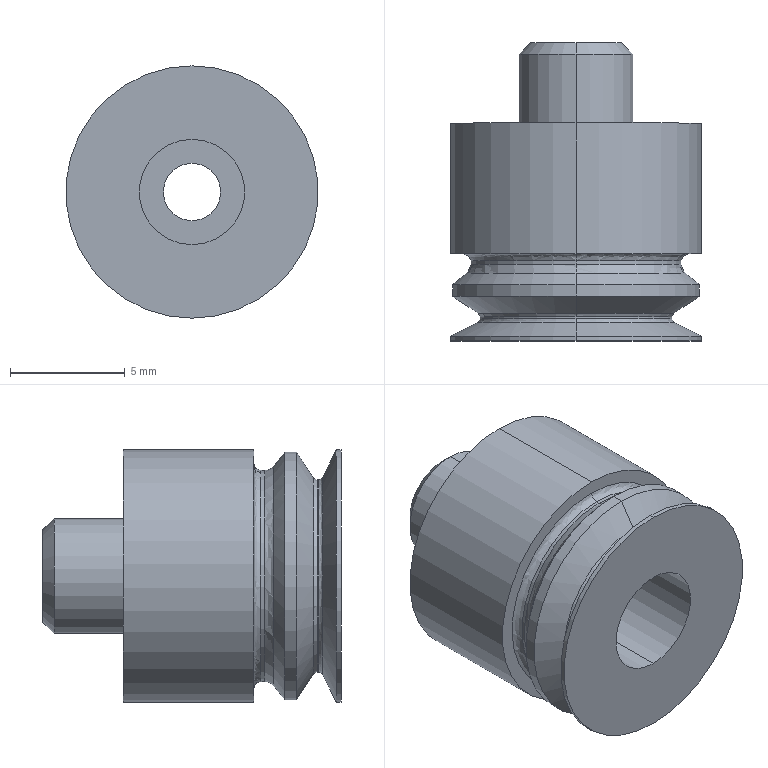Part | SolidWorks | features BaseBody 1 | 1 solid | 37 faces | box 11 x 13 x 11 mm | volume 720.123 mm3 | cylinder 16 | spline 8 | cone 8 | plane 5 | commonest cylinder face diameters 11 x4 2.5 x2 4.6 x2 5 x2 8.4 x2 9.2 x2
STEP:
#1=CARTESIAN_POINT('',(0.,-9.2,4.9));
#2=VERTEX_POINT('',#1);
#3=CARTESIAN_POINT('',(0.,-9.2,-4.9));
#4=VERTEX_POINT('',#3);
#5=CARTESIAN_POINT('',(0.,-9.2,4.9));
#6=CARTESIAN_POINT('',(0.3114,-9.2,4.9));
#7=CARTESIAN_POINT('',(0.7704,-9.2,4.857));
#8=CARTESIAN_POINT('',(1.292,-9.2,4.732));
#9=CARTESIAN_POINT('',(1.549,-9.2,4.65));
#10=CARTESIAN_POINT('',(1.677,-9.2,4.605));
#11=CARTESIAN_POINT('',(1.731,-9.2,4.584));
#12=CARTESIAN_POINT('',(1.767,-9.2,4.57));
#13=CARTESIAN_POINT('',(1.784,-9.2,4.564));
#14=CARTESIAN_POINT('',(1.957,-9.2,4.495));
#15=CARTESIAN_POINT('',(2.183,-9.2,4.393));
#16=CARTESIAN_POINT('',(2.399,-9.2,4.273));
#17=CARTESIAN_POINT('',(2.542,-9.2,4.19));
#18=CARTESIAN_POINT('',(2.611,-9.2,4.147));
#19=CARTESIAN_POINT('',(2.964,-9.2,3.916));
#20=CARTESIAN_POINT('',(3.226,-9.2,3.704));
#21=CARTESIAN_POINT('',(3.584,-9.2,3.345));
#22=CARTESIAN_POINT('',(3.753,-9.2,3.158));
#23=CARTESIAN_POINT('',(3.908,-9.2,2.958));
#24=CARTESIAN_POINT('',(4.007,-9.2,2.822));
#25=CARTESIAN_POINT('',(4.056,-9.2,2.751));
#26=CARTESIAN_POINT('',(4.192,-9.2,2.543));
#27=CARTESIAN_POINT('',(4.317,-9.2,2.329));
#28=CARTESIAN_POINT('',(4.443,-9.2,2.07));
#29=CARTESIAN_POINT('',(4.501,-9.2,1.938));
#30=CARTESIAN_POINT('',(4.525,-9.2,1.88));
#31=CARTESIAN_POINT('',(4.541,-9.2,1.842));
#32=CARTESIAN_POINT('',(4.549,-9.2,1.822));
#33=CARTESIAN_POINT('',(4.785,-9.2,1.225));
#34=CARTESIAN_POINT('',(4.9,-9.2,0.6227));
#35=CARTESIAN_POINT('',(4.9,-9.2,-0.3114));
#36=CARTESIAN_POINT('',(4.857,-9.2,-0.7704));
#37=CARTESIAN_POINT('',(4.732,-9.2,-1.292));
#38=CARTESIAN_POINT('',(4.65,-9.2,-1.549));
#39=CARTESIAN_POINT('',(4.605,-9.2,-1.677));
#40=CARTESIAN_POINT('',(4.584,-9.2,-1.731));
#41=CARTESIAN_POINT('',(4.57,-9.2,-1.767));
#42=CARTESIAN_POINT('',(4.564,-9.2,-1.784));
#43=CARTESIAN_POINT('',(4.495,-9.2,-1.957));
#44=CARTESIAN_POINT('',(4.393,-9.2,-2.183));
#45=CARTESIAN_POINT('',(4.273,-9.2,-2.399));
#46=CARTESIAN_POINT('',(4.19,-9.2,-2.542));
#47=CARTESIAN_POINT('',(4.147,-9.2,-2.611));
#48=CARTESIAN_POINT('',(3.916,-9.2,-2.964));
#49=CARTESIAN_POINT('',(3.704,-9.2,-3.226));
#50=CARTESIAN_POINT('',(3.345,-9.2,-3.584));
#51=CARTESIAN_POINT('',(3.158,-9.2,-3.753));
#52=CARTESIAN_POINT('',(2.958,-9.2,-3.908));
#53=CARTESIAN_POINT('',(2.822,-9.2,-4.007));
#54=CARTESIAN_POINT('',(2.751,-9.2,-4.056));
#55=CARTESIAN_POINT('',(2.543,-9.2,-4.192));
#56=CARTESIAN_POINT('',(2.329,-9.2,-4.317));
#57=CARTESIAN_POINT('',(2.07,-9.2,-4.443));
#58=CARTESIAN_POINT('',(1.957,-9.2,-4.493));
#59=CARTESIAN_POINT('',(1.88,-9.2,-4.525));
#60=CARTESIAN_POINT('',(1.841,-9.2,-4.541));
#61=CARTESIAN_POINT('',(1.656,-9.2,-4.614));
#62=CARTESIAN_POINT('',(1.431,-9.2,-4.691));
#63=CARTESIAN_POINT('',(1.163,-9.2,-4.761));
#64=CARTESIAN_POINT('',(1.028,-9.2,-4.791));
#65=CARTESIAN_POINT('',(0.9697,-9.2,-4.803));
#66=CARTESIAN_POINT('',(0.9307,-9.2,-4.811));
#67=CARTESIAN_POINT('',(0.91,-9.2,-4.815));
#68=CARTESIAN_POINT('',(0.5971,-9.2,-4.873));
#69=CARTESIAN_POINT('',(0.2999,-9.2,-4.9));
#70=CARTESIAN_POINT('',(0.,-9.2,-4.9));
#71=B_SPLINE_CURVE_WITH_KNOTS('',3,(#5,#6,#7,#8,#9,#10,#11,#12,#13,#14,#15,#16,#17,#18,#19,#20,#21,#22,#23,#24,#25,#26,#27,#28,#29,#30,#31,#32,#33,#34,#35,#36,#37,#38,#39,#40,#41,#42,#43,#44,#45,#46,#47,#48,#49,#50,#51,#52,#53,#54,#55,#56,#57,#58,#59,#60,#61,#62,#63,#64,#65,#66,#67,#68,#69,#70),.UNSPECIFIED.,.F.,.F.,(4,1,1,1,1,2,2,1,2,2,2,1,2,2,1,1,1,2,2,2,1,1,1,1,2,2,1,2,2,2,1,2,2,1,1,2,2,1,1,1,2,2,4),(0.5,0.5313,0.5469,0.5547,0.5586,0.5605,0.5625,0.5781,0.5859,0.5938,0.625,0.6406,0.6484,0.6563,0.6719,0.6797,0.6836,0.6855,0.6875,0.75,0.7813,0.7969,0.8047,0.8086,0.8105,0.8125,0.8281,0.8359,0.8438,0.875,0.8906,0.8984,0.9063,0.9219,0.9297,0.9336,0.9375,0.9531,0.9609,0.9648,0.9668,0.9688,1.),.UNSPECIFIED.);
#72=EDGE_CURVE('',#2,#4,#71,.T.);
#73=ORIENTED_EDGE('',*,*,#72,.F.);
#74=CARTESIAN_POINT('',(0.,-9.5,4.6));
#75=VERTEX_POINT('',#74);
#76=CARTESIAN_POINT('',(0.,-9.5,4.9));
#77=DIRECTION('',(-1.,0.,0.));
#78=DIRECTION('',(0.,0.,1.));
#79=AXIS2_PLACEMENT_3D('',#76,#77,#78);
#80=CIRCLE('',#79,0.3);
#81=EDGE_CURVE('',#2,#75,#80,.T.);
#82=ORIENTED_EDGE('',*,*,#81,.T.);
#83=CARTESIAN_POINT('',(0.,-9.5,-4.6));
#84=VERTEX_POINT('',#83);
#85=CARTESIAN_POINT('',(0.,-9.5,0.));
#86=DIRECTION('',(0.,-1.,0.));
#87=DIRECTION('',(0.,0.,-1.));
#88=AXIS2_PLACEMENT_3D('',#85,#86,#87);
#89=CIRCLE('',#88,4.6);
#90=EDGE_CURVE('',#84,#75,#89,.T.);
#91=ORIENTED_EDGE('',*,*,#90,.F.);
#92=CARTESIAN_POINT('',(0.,-9.5,-4.9));
#93=DIRECTION('',(1.,0.,0.));
#94=DIRECTION('',(0.,0.,-1.));
#95=AXIS2_PLACEMENT_3D('',#92,#93,#94);
#96=CIRCLE('',#95,0.3);
#97=EDGE_CURVE('',#4,#84,#96,.T.);
#98=ORIENTED_EDGE('',*,*,#97,.F.);
#99=EDGE_LOOP('',(#73,#82,#91,#98));
#100=FACE_OUTER_BOUND('',#99,.T.);
#101=CARTESIAN_POINT('',(0.,-9.2,-4.9));
#102=CARTESIAN_POINT('',(9.8,-9.2,-4.9));
#103=CARTESIAN_POINT('',(9.8,-9.2,4.9));
#104=CARTESIAN_POINT('',(0.,-9.2,4.9));
#105=CARTESIAN_POINT('',(0.,-9.2,-4.724));
#106=CARTESIAN_POINT('',(9.449,-9.2,-4.724));
#107=CARTESIAN_POINT('',(9.449,-9.2,4.724));
#108=CARTESIAN_POINT('',(0.,-9.2,4.724));
#109=CARTESIAN_POINT('',(0.,-9.324,-4.6));
#110=CARTESIAN_POINT('',(9.2,-9.324,-4.6));
#111=CARTESIAN_POINT('',(9.2,-9.324,4.6));
#112=CARTESIAN_POINT('',(0.,-9.324,4.6));
#113=CARTESIAN_POINT('',(0.,-9.5,-4.6));
#114=CARTESIAN_POINT('',(9.2,-9.5,-4.6));
#115=CARTESIAN_POINT('',(9.2,-9.5,4.6));
#116=CARTESIAN_POINT('',(0.,-9.5,4.6));
#117=(BOUNDED_SURFACE()B_SPLINE_SURFACE(3,3,((#101,#102,#103,#104),(#105,#106,#107,#108),(#109,#110,#111,#112),(#113,#114,#115,#116)),.UNSPECIFIED.,.F.,.F.,.T.)B_SPLINE_SURFACE_WITH_KNOTS((4,4),(4,4),(0.,1.),(0.,1.),.UNSPECIFIED.)GEOMETRIC_REPRESENTATION_ITEM()RATIONAL_B_SPLINE_SURFACE(((1.,0.3333,0.3333,1.),(0.8047,0.2682,0.2682,0.8047),(0.8047,0.2682,0.2682,0.8047),(1.,0.3333,0.3333,1.)))REPRESENTATION_ITEM('')SURFACE());
#118=ADVANCED_FACE('',(#100),#117,.F.);
#119=CARTESIAN_POINT('',(0.,-9.662,4.6));
#120=VERTEX_POINT('',#119);
#121=CARTESIAN_POINT('',(0.,-9.662,-4.6));
#122=VERTEX_POINT('',#121);
#123=CARTESIAN_POINT('',(0.,-9.662,0.));
#124=DIRECTION('',(0.,1.,0.));
#125=DIRECTION('',(0.,0.,-1.));
#126=AXIS2_PLACEMENT_3D('',#123,#124,#125);
#127=CIRCLE('',#126,4.6);
#128=EDGE_CURVE('',#120,#122,#127,.T.);
#129=ORIENTED_EDGE('',*,*,#128,.F.);
#130=CARTESIAN_POINT('',(0.,-10.05,4.785));
#131=VERTEX_POINT('',#130);
#132=CARTESIAN_POINT('',(0.,-9.662,5.1));
#133=DIRECTION('',(-1.,0.,0.));
#134=DIRECTION('',(0.,0.,1.));
#135=AXIS2_PLACEMENT_3D('',#132,#133,#134);
#136=CIRCLE('',#135,0.5);
#137=EDGE_CURVE('',#120,#131,#136,.T.);
#138=ORIENTED_EDGE('',*,*,#137,.T.);
#139=CARTESIAN_POINT('',(0.,-10.05,-4.785));
#140=VERTEX_POINT('',#139);
#141=CARTESIAN_POINT('',(0.,-10.05,0.));
#142=DIRECTION('',(0.,-1.,0.));
#143=DIRECTION('',(0.,0.,-1.));
#144=AXIS2_PLACEMENT_3D('',#141,#142,#143);
#145=CIRCLE('',#144,4.785);
#146=EDGE_CURVE('',#140,#131,#145,.T.);
#147=ORIENTED_EDGE('',*,*,#146,.F.);
#148=CARTESIAN_POINT('',(0.,-9.662,-5.1));
#149=DIRECTION('',(1.,0.,0.));
#150=DIRECTION('',(0.,0.,-1.));
#151=AXIS2_PLACEMENT_3D('',#148,#149,#150);
#152=CIRCLE('',#151,0.5);
#153=EDGE_CURVE('',#122,#140,#152,.T.);
#154=ORIENTED_EDGE('',*,*,#153,.F.);
#155=EDGE_LOOP('',(#129,#138,#147,#154));
#156=FACE_OUTER_BOUND('',#155,.T.);
#157=CARTESIAN_POINT('',(0.,-9.662,-4.6));
#158=CARTESIAN_POINT('',(9.2,-9.662,-4.6));
#159=CARTESIAN_POINT('',(9.2,-9.662,4.6));
#160=CARTESIAN_POINT('',(0.,-9.662,4.6));
#161=CARTESIAN_POINT('',(0.,-9.815,-4.6));
#162=CARTESIAN_POINT('',(9.2,-9.815,-4.6));
#163=CARTESIAN_POINT('',(9.2,-9.815,4.6));
#164=CARTESIAN_POINT('',(0.,-9.815,4.6));
#165=CARTESIAN_POINT('',(0.,-9.953,-4.666));
#166=CARTESIAN_POINT('',(9.332,-9.953,-4.666));
#167=CARTESIAN_POINT('',(9.332,-9.953,4.666));
#168=CARTESIAN_POINT('',(0.,-9.953,4.666));
#169=CARTESIAN_POINT('',(0.,-10.05,-4.785));
#170=CARTESIAN_POINT('',(9.569,-10.05,-4.785));
#171=CARTESIAN_POINT('',(9.569,-10.05,4.785));
#172=CARTESIAN_POINT('',(0.,-10.05,4.785));
#173=(BOUNDED_SURFACE()B_SPLINE_SURFACE(3,3,((#157,#158,#159,#160),(#161,#162,#163,#164),(#165,#166,#167,#168),(#169,#170,#171,#172)),.UNSPECIFIED.,.F.,.F.,.T.)B_SPLINE_SURFACE_WITH_KNOTS((4,4),(4,4),(0.,1.),(0.,1.),.UNSPECIFIED.)GEOMETRIC_REPRESENTATION_ITEM()RATIONAL_B_SPLINE_SURFACE(((1.,0.3333,0.3333,1.),(0.9353,0.3118,0.3118,0.9353),(0.9353,0.3118,0.3118,0.9353),(1.,0.3333,0.3333,1.)))REPRESENTATION_ITEM('')SURFACE());
#174=ADVANCED_FACE('',(#156),#173,.F.);
#175=CARTESIAN_POINT('',(0.,-11.788,4.289));
#176=VERTEX_POINT('',#175);
#177=CARTESIAN_POINT('',(0.,-11.788,-4.289));
#178=VERTEX_POINT('',#177);
#179=CARTESIAN_POINT('',(0.,-11.788,0.));
#180=DIRECTION('',(0.,1.,0.));
#181=DIRECTION('',(0.,0.,1.));
#182=AXIS2_PLACEMENT_3D('',#179,#180,#181);
#183=CIRCLE('',#182,4.289);
#184=EDGE_CURVE('',#176,#178,#183,.T.);
#185=ORIENTED_EDGE('',*,*,#184,.F.);
#186=CARTESIAN_POINT('',(0.,-11.954,4.2));
#187=VERTEX_POINT('',#186);
#188=CARTESIAN_POINT('',(0.,-11.954,4.4));
#189=DIRECTION('',(-1.,0.,0.));
#190=DIRECTION('',(0.,0.,1.));
#191=AXIS2_PLACEMENT_3D('',#188,#189,#190);
#192=CIRCLE('',#191,0.2);
#193=EDGE_CURVE('',#176,#187,#192,.T.);
#194=ORIENTED_EDGE('',*,*,#193,.T.);
#195=CARTESIAN_POINT('',(0.,-11.954,-4.2));
#196=VERTEX_POINT('',#195);
#197=CARTESIAN_POINT('',(0.,-11.954,0.));
#198=DIRECTION('',(0.,-1.,0.));
#199=DIRECTION('',(0.,0.,-1.));
#200=AXIS2_PLACEMENT_3D('',#197,#198,#199);
#201=CIRCLE('',#200,4.2);
#202=EDGE_CURVE('',#196,#187,#201,.T.);
#203=ORIENTED_EDGE('',*,*,#202,.F.);
#204=CARTESIAN_POINT('',(0.,-11.954,-4.4));
#205=DIRECTION('',(1.,0.,0.));
#206=DIRECTION('',(0.,0.,-1.));
#207=AXIS2_PLACEMENT_3D('',#204,#205,#206);
#208=CIRCLE('',#207,0.2);
#209=EDGE_CURVE('',#178,#196,#208,.T.);
#210=ORIENTED_EDGE('',*,*,#209,.F.);
#211=EDGE_LOOP('',(#185,#194,#203,#210));
#212=FACE_OUTER_BOUND('',#211,.T.);
#213=CARTESIAN_POINT('',(0.,-11.788,-4.289));
#214=CARTESIAN_POINT('',(8.579,-11.788,-4.289));
#215=CARTESIAN_POINT('',(8.579,-11.788,4.289));
#216=CARTESIAN_POINT('',(0.,-11.788,4.289));
#217=CARTESIAN_POINT('',(0.,-11.826,-4.232));
#218=CARTESIAN_POINT('',(8.465,-11.826,-4.232));
#219=CARTESIAN_POINT('',(8.465,-11.826,4.232));
#220=CARTESIAN_POINT('',(0.,-11.826,4.232));
#221=CARTESIAN_POINT('',(0.,-11.886,-4.2));
#222=CARTESIAN_POINT('',(8.4,-11.886,-4.2));
#223=CARTESIAN_POINT('',(8.4,-11.886,4.2));
#224=CARTESIAN_POINT('',(0.,-11.886,4.2));
#225=CARTESIAN_POINT('',(0.,-11.954,-4.2));
#226=CARTESIAN_POINT('',(8.4,-11.954,-4.2));
#227=CARTESIAN_POINT('',(8.4,-11.954,4.2));
#228=CARTESIAN_POINT('',(0.,-11.954,4.2));
#229=(BOUNDED_SURFACE()B_SPLINE_SURFACE(3,3,((#213,#214,#215,#216),(#217,#218,#219,#220),(#221,#222,#223,#224),(#225,#226,#227,#228)),.UNSPECIFIED.,.F.,.F.,.T.)B_SPLINE_SURFACE_WITH_KNOTS((4,4),(4,4),(0.,1.),(0.,1.),.UNSPECIFIED.)GEOMETRIC_REPRESENTATION_ITEM()RATIONAL_B_SPLINE_SURFACE(((1.,0.3333,0.3333,1.),(0.9209,0.307,0.307,0.9209),(0.9209,0.307,0.307,0.9209),(1.,0.3333,0.3333,1.)))REPRESENTATION_ITEM('')SURFACE());
#230=ADVANCED_FACE('',(#212),#229,.F.);
#231=CARTESIAN_POINT('',(0.,-12.026,4.2));
#232=VERTEX_POINT('',#231);
#233=CARTESIAN_POINT('',(0.,-12.026,-4.2));
#234=VERTEX_POINT('',#233);
#235=CARTESIAN_POINT('',(0.,-12.026,0.));
#236=DIRECTION('',(0.,1.,0.));
#237=DIRECTION('',(0.,0.,-1.));
#238=AXIS2_PLACEMENT_3D('',#235,#236,#237);
#239=CIRCLE('',#238,4.2);
#240=EDGE_CURVE('',#232,#234,#239,.T.);
#241=ORIENTED_EDGE('',*,*,#240,.F.);
#242=CARTESIAN_POINT('',(0.,-12.205,4.31));
#243=VERTEX_POINT('',#242);
#244=CARTESIAN_POINT('',(0.,-12.026,4.4));
#245=DIRECTION('',(-1.,0.,0.));
#246=DIRECTION('',(0.,0.,1.));
#247=AXIS2_PLACEMENT_3D('',#244,#245,#246);
#248=CIRCLE('',#247,0.2);
#249=EDGE_CURVE('',#232,#243,#248,.T.);
#250=ORIENTED_EDGE('',*,*,#249,.T.);
#251=CARTESIAN_POINT('',(0.,-12.205,-4.31));
#252=VERTEX_POINT('',#251);
#253=CARTESIAN_POINT('',(0.,-12.205,0.));
#254=DIRECTION('',(0.,-1.,0.));
#255=DIRECTION('',(0.,0.,-1.));
#256=AXIS2_PLACEMENT_3D('',#253,#254,#255);
#257=CIRCLE('',#256,4.31);
#258=EDGE_CURVE('',#252,#243,#257,.T.);
#259=ORIENTED_EDGE('',*,*,#258,.F.);
#260=CARTESIAN_POINT('',(0.,-12.026,-4.4));
#261=DIRECTION('',(1.,0.,0.));
#262=DIRECTION('',(0.,0.,-1.));
#263=AXIS2_PLACEMENT_3D('',#260,#261,#262);
#264=CIRCLE('',#263,0.2);
#265=EDGE_CURVE('',#234,#252,#264,.T.);
#266=ORIENTED_EDGE('',*,*,#265,.F.);
#267=EDGE_LOOP('',(#241,#250,#259,#266));
#268=FACE_OUTER_BOUND('',#267,.T.);
#269=CARTESIAN_POINT('',(0.,-12.026,-4.2));
#270=CARTESIAN_POINT('',(8.4,-12.026,-4.2));
#271=CARTESIAN_POINT('',(8.4,-12.026,4.2));
#272=CARTESIAN_POINT('',(0.,-12.026,4.2));
#273=CARTESIAN_POINT('',(0.,-12.104,-4.2));
#274=CARTESIAN_POINT('',(8.4,-12.104,-4.2));
#275=CARTESIAN_POINT('',(8.4,-12.104,4.2));
#276=CARTESIAN_POINT('',(0.,-12.104,4.2));
#277=CARTESIAN_POINT('',(0.,-12.17,-4.241));
#278=CARTESIAN_POINT('',(8.482,-12.17,-4.241));
#279=CARTESIAN_POINT('',(8.482,-12.17,4.241));
#280=CARTESIAN_POINT('',(0.,-12.17,4.241));
#281=CARTESIAN_POINT('',(0.,-12.205,-4.31));
#282=CARTESIAN_POINT('',(8.621,-12.205,-4.31));
#283=CARTESIAN_POINT('',(8.621,-12.205,4.31));
#284=CARTESIAN_POINT('',(0.,-12.205,4.31));
#285=(BOUNDED_SURFACE()B_SPLINE_SURFACE(3,3,((#269,#270,#271,#272),(#273,#274,#275,#276),(#277,#278,#279,#280),(#281,#282,#283,#284)),.UNSPECIFIED.,.F.,.F.,.T.)B_SPLINE_SURFACE_WITH_KNOTS((4,4),(4,4),(0.,1.),(0.,1.),.UNSPECIFIED.)GEOMETRIC_REPRESENTATION_ITEM()RATIONAL_B_SPLINE_SURFACE(((1.,0.3333,0.3333,1.),(0.9005,0.3002,0.3002,0.9005),(0.9005,0.3002,0.3002,0.9005),(1.,0.3333,0.3333,1.)))REPRESENTATION_ITEM('')SURFACE());
#286=ADVANCED_FACE('',(#268),#285,.F.);
#287=CARTESIAN_POINT('',(0.,-3.5,-5.5));
#288=VERTEX_POINT('',#287);
#289=CARTESIAN_POINT('',(0.,-3.5,5.5));
#290=VERTEX_POINT('',#289);
#291=CARTESIAN_POINT('',(0.,-3.5,0.));
#292=DIRECTION('',(0.,-1.,0.));
#293=DIRECTION('',(0.,0.,-1.));
#294=AXIS2_PLACEMENT_3D('',#291,#292,#293);
#295=CIRCLE('',#294,5.5);
#296=EDGE_CURVE('',#288,#290,#295,.T.);
#297=ORIENTED_EDGE('',*,*,#296,.T.);
#298=CARTESIAN_POINT('',(0.,-9.2,5.5));
#299=VERTEX_POINT('',#298);
#300=CARTESIAN_POINT('',(0.,-5.,5.5));
#301=DIRECTION('',(0.,-1.,0.));
#302=VECTOR('',#301,1000.);
#303=LINE('',#300,#302);
#304=EDGE_CURVE('',#290,#299,#303,.T.);
#305=ORIENTED_EDGE('',*,*,#304,.T.);
#306=CARTESIAN_POINT('',(0.,-9.2,-5.5));
#307=VERTEX_POINT('',#306);
#308=CARTESIAN_POINT('',(0.,-9.2,0.));
#309=DIRECTION('',(0.,1.,0.));
#310=DIRECTION('',(0.,0.,-1.));
#311=AXIS2_PLACEMENT_3D('',#308,#309,#310);
#312=CIRCLE('',#311,5.5);
#313=EDGE_CURVE('',#299,#307,#312,.T.);
#314=ORIENTED_EDGE('',*,*,#313,.T.);
#315=CARTESIAN_POINT('',(0.,-5.,-5.5));
#316=DIRECTION('',(0.,-1.,0.));
#317=VECTOR('',#316,1000.);
#318=LINE('',#315,#317);
#319=EDGE_CURVE('',#288,#307,#318,.T.);
#320=ORIENTED_EDGE('',*,*,#319,.F.);
#321=EDGE_LOOP('',(#297,#305,#314,#320));
#322=FACE_OUTER_BOUND('',#321,.T.);
#323=CARTESIAN_POINT('',(0.,-5.,0.));
#324=DIRECTION('',(0.,-1.,0.));
#325=DIRECTION('',(0.,0.,-1.));
#326=AXIS2_PLACEMENT_3D('',#323,#324,#325);
#327=CYLINDRICAL_SURFACE('',#326,5.5);
#328=ADVANCED_FACE('',(#322),#327,.T.);
#329=CARTESIAN_POINT('',(0.,-0.4905,-2.5));
#330=VERTEX_POINT('',#329);
#331=CARTESIAN_POINT('',(0.,-0.4905,2.5));
#332=VERTEX_POINT('',#331);
#333=CARTESIAN_POINT('',(0.,-0.4905,0.));
#334=DIRECTION('',(0.,-1.,0.));
#335=DIRECTION('',(0.,0.,-1.));
#336=AXIS2_PLACEMENT_3D('',#333,#334,#335);
#337=CIRCLE('',#336,2.5);
#338=EDGE_CURVE('',#330,#332,#337,.T.);
#339=ORIENTED_EDGE('',*,*,#338,.T.);
#340=CARTESIAN_POINT('',(0.,-3.5,2.5));
#341=VERTEX_POINT('',#340);
#342=CARTESIAN_POINT('',(0.,-5.,2.5));
#343=DIRECTION('',(0.,-1.,0.));
#344=VECTOR('',#343,1000.);
#345=LINE('',#342,#344);
#346=EDGE_CURVE('',#332,#341,#345,.T.);
#347=ORIENTED_EDGE('',*,*,#346,.T.);
#348=CARTESIAN_POINT('',(0.,-3.5,-2.5));
#349=VERTEX_POINT('',#348);
#350=CARTESIAN_POINT('',(0.,-3.5,0.));
#351=DIRECTION('',(0.,-1.,0.));
#352=DIRECTION('',(0.,0.,-1.));
#353=AXIS2_PLACEMENT_3D('',#350,#351,#352);
#354=CIRCLE('',#353,2.5);
#355=EDGE_CURVE('',#349,#341,#354,.T.);
#356=ORIENTED_EDGE('',*,*,#355,.F.);
#357=CARTESIAN_POINT('',(0.,-5.,-2.5));
#358=DIRECTION('',(0.,-1.,0.));
#359=VECTOR('',#358,1000.);
#360=LINE('',#357,#359);
#361=EDGE_CURVE('',#330,#349,#360,.T.);
#362=ORIENTED_EDGE('',*,*,#361,.F.);
#363=EDGE_LOOP('',(#339,#347,#356,#362));
#364=FACE_OUTER_BOUND('',#363,.T.);
#365=CARTESIAN_POINT('',(0.,-5.,0.));
#366=DIRECTION('',(0.,-1.,0.));
#367=DIRECTION('',(0.,0.,-1.));
#368=AXIS2_PLACEMENT_3D('',#365,#366,#367);
#369=CYLINDRICAL_SURFACE('',#368,2.5);
#370=ADVANCED_FACE('',(#364),#369,.T.);
#371=ORIENTED_EDGE('',*,*,#90,.T.);
#372=CARTESIAN_POINT('',(0.,-5.,4.6));
#373=DIRECTION('',(0.,-1.,0.));
#374=VECTOR('',#373,1000.);
#375=LINE('',#372,#374);
#376=EDGE_CURVE('',#75,#120,#375,.T.);
#377=ORIENTED_EDGE('',*,*,#376,.T.);
#378=ORIENTED_EDGE('',*,*,#128,.T.);
#379=CARTESIAN_POINT('',(0.,-5.,-4.6));
#380=DIRECTION('',(0.,-1.,0.));
#381=VECTOR('',#380,1000.);
#382=LINE('',#379,#381);
#383=EDGE_CURVE('',#84,#122,#382,.T.);
#384=ORIENTED_EDGE('',*,*,#383,.F.);
#385=EDGE_LOOP('',(#371,#377,#378,#384));
#386=FACE_OUTER_BOUND('',#385,.T.);
#387=CARTESIAN_POINT('',(0.,-5.,0.));
#388=DIRECTION('',(0.,-1.,0.));
#389=DIRECTION('',(0.,0.,-1.));
#390=AXIS2_PLACEMENT_3D('',#387,#388,#389);
#391=CYLINDRICAL_SURFACE('',#390,4.6);
#392=ADVANCED_FACE('',(#386),#391,.T.);
#393=CARTESIAN_POINT('',(0.,0.,-2.009));
#394=VERTEX_POINT('',#393);
#395=CARTESIAN_POINT('',(0.,0.,2.009));
#396=VERTEX_POINT('',#395);
#397=CARTESIAN_POINT('',(0.,0.,0.));
#398=DIRECTION('',(0.,-1.,0.));
#399=DIRECTION('',(0.,0.,-1.));
#400=AXIS2_PLACEMENT_3D('',#397,#398,#399);
#401=CIRCLE('',#400,2.009);
#402=EDGE_CURVE('',#394,#396,#401,.T.);
#403=ORIENTED_EDGE('',*,*,#402,.T.);
#404=CARTESIAN_POINT('',(0.,-0.4905,2.5));
#405=DIRECTION('',(0.,-0.7071,0.7071));
#406=VECTOR('',#405,1000.);
#407=LINE('',#404,#406);
#408=EDGE_CURVE('',#396,#332,#407,.T.);
#409=ORIENTED_EDGE('',*,*,#408,.T.);
#410=ORIENTED_EDGE('',*,*,#338,.F.);
#411=CARTESIAN_POINT('',(0.,-0.4905,-2.5));
#412=DIRECTION('',(0.,-0.7071,-0.7071));
#413=VECTOR('',#412,1000.);
#414=LINE('',#411,#413);
#415=EDGE_CURVE('',#394,#330,#414,.T.);
#416=ORIENTED_EDGE('',*,*,#415,.F.);
#417=EDGE_LOOP('',(#403,#409,#410,#416));
#418=FACE_OUTER_BOUND('',#417,.T.);
#419=CARTESIAN_POINT('',(0.,-0.4905,0.));
#420=DIRECTION('',(0.,-1.,0.));
#421=DIRECTION('',(0.,0.,-1.));
#422=AXIS2_PLACEMENT_3D('',#419,#420,#421);
#423=CONICAL_SURFACE('',#422,2.5,0.7854);
#424=ADVANCED_FACE('',(#418),#423,.T.);
#425=ORIENTED_EDGE('',*,*,#146,.T.);
#426=CARTESIAN_POINT('',(0.,-10.55,5.4));
#427=VERTEX_POINT('',#426);
#428=CARTESIAN_POINT('',(0.,-10.55,5.4));
#429=DIRECTION('',(0.,-0.6308,0.7759));
#430=VECTOR('',#429,1000.);
#431=LINE('',#428,#430);
#432=EDGE_CURVE('',#131,#427,#431,.T.);
#433=ORIENTED_EDGE('',*,*,#432,.T.);
#434=CARTESIAN_POINT('',(0.,-10.55,-5.4));
#435=VERTEX_POINT('',#434);
#436=CARTESIAN_POINT('',(0.,-10.55,0.));
#437=DIRECTION('',(0.,1.,0.));
#438=DIRECTION('',(0.,0.,-1.));
#439=AXIS2_PLACEMENT_3D('',#436,#437,#438);
#440=CIRCLE('',#439,5.4);
#441=EDGE_CURVE('',#427,#435,#440,.T.);
#442=ORIENTED_EDGE('',*,*,#441,.T.);
#443=CARTESIAN_POINT('',(0.,-10.55,-5.4));
#444=DIRECTION('',(0.,-0.6308,-0.7759));
#445=VECTOR('',#444,1000.);
#446=LINE('',#443,#445);
#447=EDGE_CURVE('',#140,#435,#446,.T.);
#448=ORIENTED_EDGE('',*,*,#447,.F.);
#449=EDGE_LOOP('',(#425,#433,#442,#448));
#450=FACE_OUTER_BOUND('',#449,.T.);
#451=CARTESIAN_POINT('',(0.,-10.55,0.));
#452=DIRECTION('',(0.,-1.,0.));
#453=DIRECTION('',(0.,0.,-1.));
#454=AXIS2_PLACEMENT_3D('',#451,#452,#453);
#455=CONICAL_SURFACE('',#454,5.4,0.8882);
#456=ADVANCED_FACE('',(#450),#455,.T.);
#457=CARTESIAN_POINT('',(0.,0.,1.25));
#458=VERTEX_POINT('',#457);
#459=CARTESIAN_POINT('',(0.,0.,-1.25));
#460=VERTEX_POINT('',#459);
#461=CARTESIAN_POINT('',(0.,0.,0.));
#462=DIRECTION('',(0.,-1.,0.));
#463=DIRECTION('',(0.,0.,-1.));
#464=AXIS2_PLACEMENT_3D('',#461,#462,#463);
#465=CIRCLE('',#464,1.25);
#466=EDGE_CURVE('',#458,#460,#465,.T.);
#467=ORIENTED_EDGE('',*,*,#466,.F.);
#468=CARTESIAN_POINT('',(0.,-3.5,1.25));
#469=VERTEX_POINT('',#468);
#470=CARTESIAN_POINT('',(0.,-5.,1.25));
#471=DIRECTION('',(0.,-1.,0.));
#472=VECTOR('',#471,1000.);
#473=LINE('',#470,#472);
#474=EDGE_CURVE('',#458,#469,#473,.T.);
#475=ORIENTED_EDGE('',*,*,#474,.T.);
#476=CARTESIAN_POINT('',(0.,-3.5,-1.25));
#477=VERTEX_POINT('',#476);
#478=CARTESIAN_POINT('',(0.,-3.5,0.));
#479=DIRECTION('',(0.,1.,0.));
#480=DIRECTION('',(0.,0.,-1.));
#481=AXIS2_PLACEMENT_3D('',#478,#479,#480);
#482=CIRCLE('',#481,1.25);
#483=EDGE_CURVE('',#477,#469,#482,.T.);
#484=ORIENTED_EDGE('',*,*,#483,.F.);
#485=CARTESIAN_POINT('',(0.,-5.,-1.25));
#486=DIRECTION('',(0.,-1.,0.));
#487=VECTOR('',#486,1000.);
#488=LINE('',#485,#487);
#489=EDGE_CURVE('',#460,#477,#488,.T.);
#490=ORIENTED_EDGE('',*,*,#489,.F.);
#491=EDGE_LOOP('',(#467,#475,#484,#490));
#492=FACE_OUTER_BOUND('',#491,.T.);
#493=CARTESIAN_POINT('',(0.,-5.,0.));
#494=DIRECTION('',(0.,-1.,0.));
#495=DIRECTION('',(0.,0.,-1.));
#496=AXIS2_PLACEMENT_3D('',#493,#494,#495);
#497=CYLINDRICAL_SURFACE('',#496,1.25);
#498=ADVANCED_FACE('',(#492),#497,.F.);
#499=ORIENTED_EDGE('',*,*,#441,.F.);
#500=CARTESIAN_POINT('',(0.,-11.05,5.4));
#501=VERTEX_POINT('',#500);
#502=CARTESIAN_POINT('',(0.,-5.,5.4));
#503=DIRECTION('',(0.,-1.,0.));
#504=VECTOR('',#503,1000.);
#505=LINE('',#502,#504);
#506=EDGE_CURVE('',#427,#501,#505,.T.);
#507=ORIENTED_EDGE('',*,*,#506,.T.);
#508=CARTESIAN_POINT('',(0.,-11.05,-5.4));
#509=VERTEX_POINT('',#508);
#510=CARTESIAN_POINT('',(0.,-11.05,0.));
#511=DIRECTION('',(0.,1.,0.));
#512=DIRECTION('',(0.,0.,-1.));
#513=AXIS2_PLACEMENT_3D('',#510,#511,#512);
#514=CIRCLE('',#513,5.4);
#515=EDGE_CURVE('',#501,#509,#514,.T.);
#516=ORIENTED_EDGE('',*,*,#515,.T.);
#517=CARTESIAN_POINT('',(0.,-5.,-5.4));
#518=DIRECTION('',(0.,-1.,0.));
#519=VECTOR('',#518,1000.);
#520=LINE('',#517,#519);
#521=EDGE_CURVE('',#435,#509,#520,.T.);
#522=ORIENTED_EDGE('',*,*,#521,.F.);
#523=EDGE_LOOP('',(#499,#507,#516,#522));
#524=FACE_OUTER_BOUND('',#523,.T.);
#525=CARTESIAN_POINT('',(0.,-5.,0.));
#526=DIRECTION('',(0.,-1.,0.));
#527=DIRECTION('',(0.,0.,-1.));
#528=AXIS2_PLACEMENT_3D('',#525,#526,#527);
#529=CYLINDRICAL_SURFACE('',#528,5.4);
#530=ADVANCED_FACE('',(#524),#529,.T.);
#531=ORIENTED_EDGE('',*,*,#184,.T.);
#532=CARTESIAN_POINT('',(0.,-11.05,-5.4));
#533=DIRECTION('',(0.,0.5533,-0.833));
#534=VECTOR('',#533,1000.);
#535=LINE('',#532,#534);
#536=EDGE_CURVE('',#178,#509,#535,.T.);
#537=ORIENTED_EDGE('',*,*,#536,.T.);
#538=ORIENTED_EDGE('',*,*,#515,.F.);
#539=CARTESIAN_POINT('',(0.,-11.05,5.4));
#540=DIRECTION('',(0.,0.5533,0.833));
#541=VECTOR('',#540,1000.);
#542=LINE('',#539,#541);
#543=EDGE_CURVE('',#176,#501,#542,.T.);
#544=ORIENTED_EDGE('',*,*,#543,.F.);
#545=EDGE_LOOP('',(#531,#537,#538,#544));
#546=FACE_OUTER_BOUND('',#545,.T.);
#547=CARTESIAN_POINT('',(0.,-11.05,0.));
#548=DIRECTION('',(0.,1.,0.));
#549=DIRECTION('',(0.,0.,1.));
#550=AXIS2_PLACEMENT_3D('',#547,#548,#549);
#551=CONICAL_SURFACE('',#550,5.4,0.9845);
#552=ADVANCED_FACE('',(#546),#551,.T.);
#553=CARTESIAN_POINT('',(0.,-3.5,2.3));
#554=VERTEX_POINT('',#553);
#555=CARTESIAN_POINT('',(0.,-3.5,-2.3));
#556=VERTEX_POINT('',#555);
#557=CARTESIAN_POINT('',(0.,-3.5,0.));
#558=DIRECTION('',(0.,-1.,0.));
#559=DIRECTION('',(0.,0.,-1.));
#560=AXIS2_PLACEMENT_3D('',#557,#558,#559);
#561=CIRCLE('',#560,2.3);
#562=EDGE_CURVE('',#554,#556,#561,.T.);
#563=ORIENTED_EDGE('',*,*,#562,.F.);
#564=CARTESIAN_POINT('',(0.,-13.,2.3));
#565=VERTEX_POINT('',#564);
#566=CARTESIAN_POINT('',(0.,-5.,2.3));
#567=DIRECTION('',(0.,-1.,0.));
#568=VECTOR('',#567,1000.);
#569=LINE('',#566,#568);
#570=EDGE_CURVE('',#554,#565,#569,.T.);
#571=ORIENTED_EDGE('',*,*,#570,.T.);
#572=CARTESIAN_POINT('',(0.,-13.,-2.3));
#573=VERTEX_POINT('',#572);
#574=CARTESIAN_POINT('',(0.,-13.,0.));
#575=DIRECTION('',(0.,1.,0.));
#576=DIRECTION('',(0.,0.,-1.));
#577=AXIS2_PLACEMENT_3D('',#574,#575,#576);
#578=CIRCLE('',#577,2.3);
#579=EDGE_CURVE('',#573,#565,#578,.T.);
#580=ORIENTED_EDGE('',*,*,#579,.F.);
#581=CARTESIAN_POINT('',(0.,-5.,-2.3));
#582=DIRECTION('',(0.,-1.,0.));
#583=VECTOR('',#582,1000.);
#584=LINE('',#581,#583);
#585=EDGE_CURVE('',#556,#573,#584,.T.);
#586=ORIENTED_EDGE('',*,*,#585,.F.);
#587=EDGE_LOOP('',(#563,#571,#580,#586));
#588=FACE_OUTER_BOUND('',#587,.T.);
#589=CARTESIAN_POINT('',(0.,-5.,0.));
#590=DIRECTION('',(0.,-1.,0.));
#591=DIRECTION('',(0.,0.,-1.));
#592=AXIS2_PLACEMENT_3D('',#589,#590,#591);
#593=CYLINDRICAL_SURFACE('',#592,2.3);
#594=ADVANCED_FACE('',(#588),#593,.F.);
#595=ORIENTED_EDGE('',*,*,#202,.T.);
#596=CARTESIAN_POINT('',(0.,-5.,4.2));
#597=DIRECTION('',(0.,-1.,0.));
#598=VECTOR('',#597,1000.);
#599=LINE('',#596,#598);
#600=EDGE_CURVE('',#187,#232,#599,.T.);
#601=ORIENTED_EDGE('',*,*,#600,.T.);
#602=ORIENTED_EDGE('',*,*,#240,.T.);
#603=CARTESIAN_POINT('',(0.,-5.,-4.2));
#604=DIRECTION('',(0.,-1.,0.));
#605=VECTOR('',#604,1000.);
#606=LINE('',#603,#605);
#607=EDGE_CURVE('',#196,#234,#606,.T.);
#608=ORIENTED_EDGE('',*,*,#607,.F.);
#609=EDGE_LOOP('',(#595,#601,#602,#608));
#610=FACE_OUTER_BOUND('',#609,.T.);
#611=CARTESIAN_POINT('',(0.,-5.,0.));
#612=DIRECTION('',(0.,-1.,0.));
#613=DIRECTION('',(0.,0.,-1.));
#614=AXIS2_PLACEMENT_3D('',#611,#612,#613);
#615=CYLINDRICAL_SURFACE('',#614,4.2);
#616=ADVANCED_FACE('',(#610),#615,.T.);
#617=CARTESIAN_POINT('',(0.,-12.8,-5.5));
#618=VERTEX_POINT('',#617);
#619=CARTESIAN_POINT('',(0.,-12.8,5.5));
#620=VERTEX_POINT('',#619);
#621=CARTESIAN_POINT('',(0.,-12.8,0.));
#622=DIRECTION('',(0.,-1.,0.));
#623=DIRECTION('',(0.,0.,-1.));
#624=AXIS2_PLACEMENT_3D('',#621,#622,#623);
#625=CIRCLE('',#624,5.5);
#626=EDGE_CURVE('',#618,#620,#625,.T.);
#627=ORIENTED_EDGE('',*,*,#626,.T.);
#628=CARTESIAN_POINT('',(0.,-13.,5.5));
#629=VERTEX_POINT('',#628);
#630=CARTESIAN_POINT('',(0.,-5.,5.5));
#631=DIRECTION('',(0.,-1.,0.));
#632=VECTOR('',#631,1000.);
#633=LINE('',#630,#632);
#634=EDGE_CURVE('',#620,#629,#633,.T.);
#635=ORIENTED_EDGE('',*,*,#634,.T.);
#636=CARTESIAN_POINT('',(0.,-13.,-5.5));
#637=VERTEX_POINT('',#636);
#638=CARTESIAN_POINT('',(0.,-13.,0.));
#639=DIRECTION('',(0.,-1.,0.));
#640=DIRECTION('',(0.,0.,-1.));
#641=AXIS2_PLACEMENT_3D('',#638,#639,#640);
#642=CIRCLE('',#641,5.5);
#643=EDGE_CURVE('',#637,#629,#642,.T.);
#644=ORIENTED_EDGE('',*,*,#643,.F.);
#645=CARTESIAN_POINT('',(0.,-5.,-5.5));
#646=DIRECTION('',(0.,-1.,0.));
#647=VECTOR('',#646,1000.);
#648=LINE('',#645,#647);
#649=EDGE_CURVE('',#618,#637,#648,.T.);
#650=ORIENTED_EDGE('',*,*,#649,.F.);
#651=EDGE_LOOP('',(#627,#635,#644,#650));
#652=FACE_OUTER_BOUND('',#651,.T.);
#653=CARTESIAN_POINT('',(0.,-5.,0.));
#654=DIRECTION('',(0.,-1.,0.));
#655=DIRECTION('',(0.,0.,-1.));
#656=AXIS2_PLACEMENT_3D('',#653,#654,#655);
#657=CYLINDRICAL_SURFACE('',#656,5.5);
#658=ADVANCED_FACE('',(#652),#657,.T.);
#659=ORIENTED_EDGE('',*,*,#258,.T.);
#660=CARTESIAN_POINT('',(0.,-12.8,5.5));
#661=DIRECTION('',(0.,-0.4475,0.8943));
#662=VECTOR('',#661,1000.);
#663=LINE('',#660,#662);
#664=EDGE_CURVE('',#243,#620,#663,.T.);
#665=ORIENTED_EDGE('',*,*,#664,.T.);
#666=ORIENTED_EDGE('',*,*,#626,.F.);
#667=CARTESIAN_POINT('',(0.,-12.8,-5.5));
#668=DIRECTION('',(0.,-0.4475,-0.8943));
#669=VECTOR('',#668,1000.);
#670=LINE('',#667,#669);
#671=EDGE_CURVE('',#252,#618,#670,.T.);
#672=ORIENTED_EDGE('',*,*,#671,.F.);
#673=EDGE_LOOP('',(#659,#665,#666,#672));
#674=FACE_OUTER_BOUND('',#673,.T.);
#675=CARTESIAN_POINT('',(0.,-12.8,0.));
#676=DIRECTION('',(0.,-1.,0.));
#677=DIRECTION('',(0.,0.,-1.));
#678=AXIS2_PLACEMENT_3D('',#675,#676,#677);
#679=CONICAL_SURFACE('',#678,5.5,1.107);
#680=ADVANCED_FACE('',(#674),#679,.T.);
#681=ORIENTED_EDGE('',*,*,#304,.F.);
#682=CARTESIAN_POINT('',(0.,-3.5,0.));
#683=DIRECTION('',(0.,-1.,0.));
#684=DIRECTION('',(0.,0.,-1.));
#685=AXIS2_PLACEMENT_3D('',#682,#683,#684);
#686=CIRCLE('',#685,5.5);
#687=EDGE_CURVE('',#290,#288,#686,.T.);
#688=ORIENTED_EDGE('',*,*,#687,.T.);
#689=ORIENTED_EDGE('',*,*,#319,.T.);
#690=CARTESIAN_POINT('',(0.,-9.2,0.));
#691=DIRECTION('',(0.,1.,0.));
#692=DIRECTION('',(0.,0.,-1.));
#693=AXIS2_PLACEMENT_3D('',#690,#691,#692);
#694=CIRCLE('',#693,5.5);
#695=EDGE_CURVE('',#307,#299,#694,.T.);
#696=ORIENTED_EDGE('',*,*,#695,.T.);
#697=EDGE_LOOP('',(#681,#688,#689,#696));
#698=FACE_OUTER_BOUND('',#697,.T.);
#699=CARTESIAN_POINT('',(0.,-5.,0.));
#700=DIRECTION('',(0.,-1.,0.));
#701=DIRECTION('',(0.,0.,-1.));
#702=AXIS2_PLACEMENT_3D('',#699,#700,#701);
#703=CYLINDRICAL_SURFACE('',#702,5.5);
#704=ADVANCED_FACE('',(#698),#703,.T.);
#705=CARTESIAN_POINT('',(0.,-9.2,-4.9));
#706=CARTESIAN_POINT('',(-0.3115,-9.2,-4.9));
#707=CARTESIAN_POINT('',(-0.7705,-9.2,-4.857));
#708=CARTESIAN_POINT('',(-1.292,-9.2,-4.732));
#709=CARTESIAN_POINT('',(-1.549,-9.2,-4.65));
#710=CARTESIAN_POINT('',(-1.677,-9.2,-4.605));
#711=CARTESIAN_POINT('',(-1.731,-9.2,-4.584));
#712=CARTESIAN_POINT('',(-1.767,-9.2,-4.57));
#713=CARTESIAN_POINT('',(-1.784,-9.2,-4.564));
#714=CARTESIAN_POINT('',(-1.957,-9.2,-4.495));
#715=CARTESIAN_POINT('',(-2.183,-9.2,-4.393));
#716=CARTESIAN_POINT('',(-2.399,-9.2,-4.273));
#717=CARTESIAN_POINT('',(-2.542,-9.2,-4.19));
#718=CARTESIAN_POINT('',(-2.611,-9.2,-4.147));
#719=CARTESIAN_POINT('',(-2.964,-9.2,-3.916));
#720=CARTESIAN_POINT('',(-3.226,-9.2,-3.704));
#721=CARTESIAN_POINT('',(-3.584,-9.2,-3.345));
#722=CARTESIAN_POINT('',(-3.753,-9.2,-3.158));
#723=CARTESIAN_POINT('',(-3.908,-9.2,-2.958));
#724=CARTESIAN_POINT('',(-4.007,-9.2,-2.822));
#725=CARTESIAN_POINT('',(-4.056,-9.2,-2.751));
#726=CARTESIAN_POINT('',(-4.192,-9.2,-2.543));
#727=CARTESIAN_POINT('',(-4.317,-9.2,-2.329));
#728=CARTESIAN_POINT('',(-4.443,-9.2,-2.07));
#729=CARTESIAN_POINT('',(-4.501,-9.2,-1.938));
#730=CARTESIAN_POINT('',(-4.525,-9.2,-1.88));
#731=CARTESIAN_POINT('',(-4.541,-9.2,-1.842));
#732=CARTESIAN_POINT('',(-4.549,-9.2,-1.822));
#733=CARTESIAN_POINT('',(-4.785,-9.2,-1.225));
#734=CARTESIAN_POINT('',(-4.9,-9.2,-0.6227));
#735=CARTESIAN_POINT('',(-4.9,-9.2,0.3114));
#736=CARTESIAN_POINT('',(-4.857,-9.2,0.7704));
#737=CARTESIAN_POINT('',(-4.732,-9.2,1.292));
#738=CARTESIAN_POINT('',(-4.65,-9.2,1.549));
#739=CARTESIAN_POINT('',(-4.605,-9.2,1.677));
#740=CARTESIAN_POINT('',(-4.584,-9.2,1.731));
#741=CARTESIAN_POINT('',(-4.57,-9.2,1.767));
#742=CARTESIAN_POINT('',(-4.564,-9.2,1.784));
#743=CARTESIAN_POINT('',(-4.495,-9.2,1.957));
#744=CARTESIAN_POINT('',(-4.393,-9.2,2.183));
#745=CARTESIAN_POINT('',(-4.273,-9.2,2.399));
#746=CARTESIAN_POINT('',(-4.19,-9.2,2.542));
#747=CARTESIAN_POINT('',(-4.147,-9.2,2.611));
#748=CARTESIAN_POINT('',(-3.916,-9.2,2.964));
#749=CARTESIAN_POINT('',(-3.704,-9.2,3.226));
#750=CARTESIAN_POINT('',(-3.345,-9.2,3.584));
#751=CARTESIAN_POINT('',(-3.158,-9.2,3.753));
#752=CARTESIAN_POINT('',(-2.958,-9.2,3.908));
#753=CARTESIAN_POINT('',(-2.822,-9.2,4.007));
#754=CARTESIAN_POINT('',(-2.751,-9.2,4.056));
#755=CARTESIAN_POINT('',(-2.543,-9.2,4.192));
#756=CARTESIAN_POINT('',(-2.329,-9.2,4.317));
#757=CARTESIAN_POINT('',(-2.07,-9.2,4.443));
#758=CARTESIAN_POINT('',(-1.938,-9.2,4.501));
#759=CARTESIAN_POINT('',(-1.88,-9.2,4.525));
#760=CARTESIAN_POINT('',(-1.842,-9.2,4.541));
#761=CARTESIAN_POINT('',(-1.822,-9.2,4.549));
#762=CARTESIAN_POINT('',(-1.225,-9.2,4.785));
#763=CARTESIAN_POINT('',(-0.6227,-9.2,4.9));
#764=CARTESIAN_POINT('',(0.,-9.2,4.9));
#765=B_SPLINE_CURVE_WITH_KNOTS('',3,(#705,#706,#707,#708,#709,#710,#711,#712,#713,#714,#715,#716,#717,#718,#719,#720,#721,#722,#723,#724,#725,#726,#727,#728,#729,#730,#731,#732,#733,#734,#735,#736,#737,#738,#739,#740,#741,#742,#743,#744,#745,#746,#747,#748,#749,#750,#751,#752,#753,#754,#755,#756,#757,#758,#759,#760,#761,#762,#763,#764),.UNSPECIFIED.,.F.,.F.,(4,1,1,1,1,2,2,1,2,2,2,1,2,2,1,1,1,2,2,2,1,1,1,1,2,2,1,2,2,2,1,2,2,1,1,1,2,2,4),(0.,0.03125,0.04687,0.05469,0.05859,0.06055,0.0625,0.07812,0.08594,0.09375,0.125,0.1406,0.1484,0.1562,0.1719,0.1797,0.1836,0.1855,0.1875,0.25,0.2812,0.2969,0.3047,0.3086,0.3105,0.3125,0.3281,0.3359,0.3437,0.375,0.3906,0.3984,0.4062,0.4219,0.4297,0.4336,0.4355,0.4375,0.5),.UNSPECIFIED.);
#766=EDGE_CURVE('',#4,#2,#765,.T.);
#767=ORIENTED_EDGE('',*,*,#766,.T.);
#768=ORIENTED_EDGE('',*,*,#72,.T.);
#769=EDGE_LOOP('',(#767,#768));
#770=FACE_BOUND('',#769,.T.);
#771=ORIENTED_EDGE('',*,*,#695,.F.);
#772=ORIENTED_EDGE('',*,*,#313,.F.);
#773=EDGE_LOOP('',(#771,#772));
#774=FACE_OUTER_BOUND('',#773,.T.);
#775=CARTESIAN_POINT('',(4.9,-9.2,0.));
#776=DIRECTION('',(0.,-1.,0.));
#777=DIRECTION('',(0.,0.,-1.));
#778=AXIS2_PLACEMENT_3D('',#775,#776,#777);
#779=PLANE('',#778);
#780=ADVANCED_FACE('',(#770,#774),#779,.T.);
#781=ORIENTED_EDGE('',*,*,#296,.F.);
#782=ORIENTED_EDGE('',*,*,#687,.F.);
#783=EDGE_LOOP('',(#781,#782));
#784=FACE_OUTER_BOUND('',#783,.T.);
#785=ORIENTED_EDGE('',*,*,#355,.T.);
#786=CARTESIAN_POINT('',(0.,-3.5,0.));
#787=DIRECTION('',(0.,-1.,0.));
#788=DIRECTION('',(0.,0.,-1.));
#789=AXIS2_PLACEMENT_3D('',#786,#787,#788);
#790=CIRCLE('',#789,2.5);
#791=EDGE_CURVE('',#341,#349,#790,.T.);
#792=ORIENTED_EDGE('',*,*,#791,.T.);
#793=EDGE_LOOP('',(#785,#792));
#794=FACE_BOUND('',#793,.T.);
#795=CARTESIAN_POINT('',(5.5,-3.5,0.));
#796=DIRECTION('',(0.,1.,0.));
#797=DIRECTION('',(0.,0.,1.));
#798=AXIS2_PLACEMENT_3D('',#795,#796,#797);
#799=PLANE('',#798);
#800=ADVANCED_FACE('',(#784,#794),#799,.T.);
#801=ORIENTED_EDGE('',*,*,#81,.F.);
#802=ORIENTED_EDGE('',*,*,#766,.F.);
#803=ORIENTED_EDGE('',*,*,#97,.T.);
#804=CARTESIAN_POINT('',(0.,-9.5,0.));
#805=DIRECTION('',(0.,-1.,0.));
#806=DIRECTION('',(0.,0.,-1.));
#807=AXIS2_PLACEMENT_3D('',#804,#805,#806);
#808=CIRCLE('',#807,4.6);
#809=EDGE_CURVE('',#75,#84,#808,.T.);
#810=ORIENTED_EDGE('',*,*,#809,.F.);
#811=EDGE_LOOP('',(#801,#802,#803,#810));
#812=FACE_OUTER_BOUND('',#811,.T.);
#813=CARTESIAN_POINT('',(0.,-9.2,4.9));
#814=CARTESIAN_POINT('',(-9.8,-9.2,4.9));
#815=CARTESIAN_POINT('',(-9.8,-9.2,-4.9));
#816=CARTESIAN_POINT('',(0.,-9.2,-4.9));
#817=CARTESIAN_POINT('',(0.,-9.2,4.724));
#818=CARTESIAN_POINT('',(-9.449,-9.2,4.724));
#819=CARTESIAN_POINT('',(-9.449,-9.2,-4.724));
#820=CARTESIAN_POINT('',(0.,-9.2,-4.724));
#821=CARTESIAN_POINT('',(0.,-9.324,4.6));
#822=CARTESIAN_POINT('',(-9.2,-9.324,4.6));
#823=CARTESIAN_POINT('',(-9.2,-9.324,-4.6));
#824=CARTESIAN_POINT('',(0.,-9.324,-4.6));
#825=CARTESIAN_POINT('',(0.,-9.5,4.6));
#826=CARTESIAN_POINT('',(-9.2,-9.5,4.6));
#827=CARTESIAN_POINT('',(-9.2,-9.5,-4.6));
#828=CARTESIAN_POINT('',(0.,-9.5,-4.6));
#829=(BOUNDED_SURFACE()B_SPLINE_SURFACE(3,3,((#813,#814,#815,#816),(#817,#818,#819,#820),(#821,#822,#823,#824),(#825,#826,#827,#828)),.UNSPECIFIED.,.F.,.F.,.T.)B_SPLINE_SURFACE_WITH_KNOTS((4,4),(4,4),(0.,1.),(0.,1.),.UNSPECIFIED.)GEOMETRIC_REPRESENTATION_ITEM()RATIONAL_B_SPLINE_SURFACE(((1.,0.3333,0.3333,1.),(0.8047,0.2682,0.2682,0.8047),(0.8047,0.2682,0.2682,0.8047),(1.,0.3333,0.3333,1.)))REPRESENTATION_ITEM('')SURFACE());
#830=ADVANCED_FACE('',(#812),#829,.F.);
#831=ORIENTED_EDGE('',*,*,#346,.F.);
#832=CARTESIAN_POINT('',(0.,-0.4905,0.));
#833=DIRECTION('',(0.,-1.,0.));
#834=DIRECTION('',(0.,0.,-1.));
#835=AXIS2_PLACEMENT_3D('',#832,#833,#834);
#836=CIRCLE('',#835,2.5);
#837=EDGE_CURVE('',#332,#330,#836,.T.);
#838=ORIENTED_EDGE('',*,*,#837,.T.);
#839=ORIENTED_EDGE('',*,*,#361,.T.);
#840=ORIENTED_EDGE('',*,*,#791,.F.);
#841=EDGE_LOOP('',(#831,#838,#839,#840));
#842=FACE_OUTER_BOUND('',#841,.T.);
#843=CARTESIAN_POINT('',(0.,-5.,0.));
#844=DIRECTION('',(0.,-1.,0.));
#845=DIRECTION('',(0.,0.,-1.));
#846=AXIS2_PLACEMENT_3D('',#843,#844,#845);
#847=CYLINDRICAL_SURFACE('',#846,2.5);
#848=ADVANCED_FACE('',(#842),#847,.T.);
#849=ORIENTED_EDGE('',*,*,#376,.F.);
#850=ORIENTED_EDGE('',*,*,#809,.T.);
#851=ORIENTED_EDGE('',*,*,#383,.T.);
#852=CARTESIAN_POINT('',(0.,-9.662,0.));
#853=DIRECTION('',(0.,1.,0.));
#854=DIRECTION('',(0.,0.,-1.));
#855=AXIS2_PLACEMENT_3D('',#852,#853,#854);
#856=CIRCLE('',#855,4.6);
#857=EDGE_CURVE('',#122,#120,#856,.T.);
#858=ORIENTED_EDGE('',*,*,#857,.T.);
#859=EDGE_LOOP('',(#849,#850,#851,#858));
#860=FACE_OUTER_BOUND('',#859,.T.);
#861=CARTESIAN_POINT('',(0.,-5.,0.));
#862=DIRECTION('',(0.,-1.,0.));
#863=DIRECTION('',(0.,0.,-1.));
#864=AXIS2_PLACEMENT_3D('',#861,#862,#863);
#865=CYLINDRICAL_SURFACE('',#864,4.6);
#866=ADVANCED_FACE('',(#860),#865,.T.);
#867=ORIENTED_EDGE('',*,*,#408,.F.);
#868=CARTESIAN_POINT('',(0.,0.,0.));
#869=DIRECTION('',(0.,-1.,0.));
#870=DIRECTION('',(0.,0.,-1.));
#871=AXIS2_PLACEMENT_3D('',#868,#869,#870);
#872=CIRCLE('',#871,2.009);
#873=EDGE_CURVE('',#396,#394,#872,.T.);
#874=ORIENTED_EDGE('',*,*,#873,.T.);
#875=ORIENTED_EDGE('',*,*,#415,.T.);
#876=ORIENTED_EDGE('',*,*,#837,.F.);
#877=EDGE_LOOP('',(#867,#874,#875,#876));
#878=FACE_OUTER_BOUND('',#877,.T.);
#879=CARTESIAN_POINT('',(0.,-0.4905,0.));
#880=DIRECTION('',(0.,-1.,0.));
#881=DIRECTION('',(0.,0.,-1.));
#882=AXIS2_PLACEMENT_3D('',#879,#880,#881);
#883=CONICAL_SURFACE('',#882,2.5,0.7854);
#884=ADVANCED_FACE('',(#878),#883,.T.);
#885=ORIENTED_EDGE('',*,*,#137,.F.);
#886=ORIENTED_EDGE('',*,*,#857,.F.);
#887=ORIENTED_EDGE('',*,*,#153,.T.);
#888=CARTESIAN_POINT('',(0.,-10.05,0.));
#889=DIRECTION('',(0.,-1.,0.));
#890=DIRECTION('',(0.,0.,-1.));
#891=AXIS2_PLACEMENT_3D('',#888,#889,#890);
#892=CIRCLE('',#891,4.785);
#893=EDGE_CURVE('',#131,#140,#892,.T.);
#894=ORIENTED_EDGE('',*,*,#893,.F.);
#895=EDGE_LOOP('',(#885,#886,#887,#894));
#896=FACE_OUTER_BOUND('',#895,.T.);
#897=CARTESIAN_POINT('',(0.,-9.662,4.6));
#898=CARTESIAN_POINT('',(-9.2,-9.662,4.6));
#899=CARTESIAN_POINT('',(-9.2,-9.662,-4.6));
#900=CARTESIAN_POINT('',(0.,-9.662,-4.6));
#901=CARTESIAN_POINT('',(0.,-9.815,4.6));
#902=CARTESIAN_POINT('',(-9.2,-9.815,4.6));
#903=CARTESIAN_POINT('',(-9.2,-9.815,-4.6));
#904=CARTESIAN_POINT('',(0.,-9.815,-4.6));
#905=CARTESIAN_POINT('',(0.,-9.953,4.666));
#906=CARTESIAN_POINT('',(-9.332,-9.953,4.666));
#907=CARTESIAN_POINT('',(-9.332,-9.953,-4.666));
#908=CARTESIAN_POINT('',(0.,-9.953,-4.666));
#909=CARTESIAN_POINT('',(0.,-10.05,4.785));
#910=CARTESIAN_POINT('',(-9.569,-10.05,4.785));
#911=CARTESIAN_POINT('',(-9.569,-10.05,-4.785));
#912=CARTESIAN_POINT('',(0.,-10.05,-4.785));
#913=(BOUNDED_SURFACE()B_SPLINE_SURFACE(3,3,((#897,#898,#899,#900),(#901,#902,#903,#904),(#905,#906,#907,#908),(#909,#910,#911,#912)),.UNSPECIFIED.,.F.,.F.,.T.)B_SPLINE_SURFACE_WITH_KNOTS((4,4),(4,4),(0.,1.),(0.,1.),.UNSPECIFIED.)GEOMETRIC_REPRESENTATION_ITEM()RATIONAL_B_SPLINE_SURFACE(((1.,0.3333,0.3333,1.),(0.9353,0.3118,0.3118,0.9353),(0.9353,0.3118,0.3118,0.9353),(1.,0.3333,0.3333,1.)))REPRESENTATION_ITEM('')SURFACE());
#914=ADVANCED_FACE('',(#896),#913,.F.);
#915=ORIENTED_EDGE('',*,*,#402,.F.);
#916=ORIENTED_EDGE('',*,*,#873,.F.);
#917=EDGE_LOOP('',(#915,#916));
#918=FACE_OUTER_BOUND('',#917,.T.);
#919=CARTESIAN_POINT('',(0.,0.,0.));
#920=DIRECTION('',(0.,-1.,0.));
#921=DIRECTION('',(0.,0.,-1.));
#922=AXIS2_PLACEMENT_3D('',#919,#920,#921);
#923=CIRCLE('',#922,1.25);
#924=EDGE_CURVE('',#460,#458,#923,.T.);
#925=ORIENTED_EDGE('',*,*,#924,.T.);
#926=ORIENTED_EDGE('',*,*,#466,.T.);
#927=EDGE_LOOP('',(#925,#926));
#928=FACE_BOUND('',#927,.T.);
#929=CARTESIAN_POINT('',(2.01,0.,0.));
#930=DIRECTION('',(0.,1.,0.));
#931=DIRECTION('',(0.,0.,1.));
#932=AXIS2_PLACEMENT_3D('',#929,#930,#931);
#933=PLANE('',#932);
#934=ADVANCED_FACE('',(#918,#928),#933,.T.);
#935=ORIENTED_EDGE('',*,*,#432,.F.);
#936=ORIENTED_EDGE('',*,*,#893,.T.);
#937=ORIENTED_EDGE('',*,*,#447,.T.);
#938=CARTESIAN_POINT('',(0.,-10.55,0.));
#939=DIRECTION('',(0.,1.,0.));
#940=DIRECTION('',(0.,0.,-1.));
#941=AXIS2_PLACEMENT_3D('',#938,#939,#940);
#942=CIRCLE('',#941,5.4);
#943=EDGE_CURVE('',#435,#427,#942,.T.);
#944=ORIENTED_EDGE('',*,*,#943,.T.);
#945=EDGE_LOOP('',(#935,#936,#937,#944));
#946=FACE_OUTER_BOUND('',#945,.T.);
#947=CARTESIAN_POINT('',(0.,-10.55,0.));
#948=DIRECTION('',(0.,-1.,0.));
#949=DIRECTION('',(0.,0.,-1.));
#950=AXIS2_PLACEMENT_3D('',#947,#948,#949);
#951=CONICAL_SURFACE('',#950,5.4,0.8882);
#952=ADVANCED_FACE('',(#946),#951,.T.);
#953=ORIENTED_EDGE('',*,*,#474,.F.);
#954=ORIENTED_EDGE('',*,*,#924,.F.);
#955=ORIENTED_EDGE('',*,*,#489,.T.);
#956=CARTESIAN_POINT('',(0.,-3.5,0.));
#957=DIRECTION('',(0.,1.,0.));
#958=DIRECTION('',(0.,0.,-1.));
#959=AXIS2_PLACEMENT_3D('',#956,#957,#958);
#960=CIRCLE('',#959,1.25);
#961=EDGE_CURVE('',#469,#477,#960,.T.);
#962=ORIENTED_EDGE('',*,*,#961,.F.);
#963=EDGE_LOOP('',(#953,#954,#955,#962));
#964=FACE_OUTER_BOUND('',#963,.T.);
#965=CARTESIAN_POINT('',(0.,-5.,0.));
#966=DIRECTION('',(0.,-1.,0.));
#967=DIRECTION('',(0.,0.,-1.));
#968=AXIS2_PLACEMENT_3D('',#965,#966,#967);
#969=CYLINDRICAL_SURFACE('',#968,1.25);
#970=ADVANCED_FACE('',(#964),#969,.F.);
#971=ORIENTED_EDGE('',*,*,#506,.F.);
#972=ORIENTED_EDGE('',*,*,#943,.F.);
#973=ORIENTED_EDGE('',*,*,#521,.T.);
#974=CARTESIAN_POINT('',(0.,-11.05,0.));
#975=DIRECTION('',(0.,1.,0.));
#976=DIRECTION('',(0.,0.,-1.));
#977=AXIS2_PLACEMENT_3D('',#974,#975,#976);
#978=CIRCLE('',#977,5.4);
#979=EDGE_CURVE('',#509,#501,#978,.T.);
#980=ORIENTED_EDGE('',*,*,#979,.T.);
#981=EDGE_LOOP('',(#971,#972,#973,#980));
#982=FACE_OUTER_BOUND('',#981,.T.);
#983=CARTESIAN_POINT('',(0.,-5.,0.));
#984=DIRECTION('',(0.,-1.,0.));
#985=DIRECTION('',(0.,0.,-1.));
#986=AXIS2_PLACEMENT_3D('',#983,#984,#985);
#987=CYLINDRICAL_SURFACE('',#986,5.4);
#988=ADVANCED_FACE('',(#982),#987,.T.);
#989=ORIENTED_EDGE('',*,*,#483,.T.);
#990=ORIENTED_EDGE('',*,*,#961,.T.);
#991=EDGE_LOOP('',(#989,#990));
#992=FACE_BOUND('',#991,.T.);
#993=CARTESIAN_POINT('',(0.,-3.5,0.));
#994=DIRECTION('',(0.,-1.,0.));
#995=DIRECTION('',(0.,0.,-1.));
#996=AXIS2_PLACEMENT_3D('',#993,#994,#995);
#997=CIRCLE('',#996,2.3);
#998=EDGE_CURVE('',#556,#554,#997,.T.);
#999=ORIENTED_EDGE('',*,*,#998,.T.);
#1000=ORIENTED_EDGE('',*,*,#562,.T.);
#1001=EDGE_LOOP('',(#999,#1000));
#1002=FACE_OUTER_BOUND('',#1001,.T.);
#1003=CARTESIAN_POINT('',(1.25,-3.5,0.));
#1004=DIRECTION('',(0.,-1.,0.));
#1005=DIRECTION('',(0.,0.,-1.));
#1006=AXIS2_PLACEMENT_3D('',#1003,#1004,#1005);
#1007=PLANE('',#1006);
#1008=ADVANCED_FACE('',(#992,#1002),#1007,.T.);
#1009=ORIENTED_EDGE('',*,*,#536,.F.);
#1010=CARTESIAN_POINT('',(0.,-11.788,0.));
#1011=DIRECTION('',(0.,1.,0.));
#1012=DIRECTION('',(0.,0.,1.));
#1013=AXIS2_PLACEMENT_3D('',#1010,#1011,#1012);
#1014=CIRCLE('',#1013,4.289);
#1015=EDGE_CURVE('',#178,#176,#1014,.T.);
#1016=ORIENTED_EDGE('',*,*,#1015,.T.);
#1017=ORIENTED_EDGE('',*,*,#543,.T.);
#1018=ORIENTED_EDGE('',*,*,#979,.F.);
#1019=EDGE_LOOP('',(#1009,#1016,#1017,#1018));
#1020=FACE_OUTER_BOUND('',#1019,.T.);
#1021=CARTESIAN_POINT('',(0.,-11.05,0.));
#1022=DIRECTION('',(0.,1.,0.));
#1023=DIRECTION('',(0.,0.,1.));
#1024=AXIS2_PLACEMENT_3D('',#1021,#1022,#1023);
#1025=CONICAL_SURFACE('',#1024,5.4,0.9845);
#1026=ADVANCED_FACE('',(#1020),#1025,.T.);
#1027=ORIENTED_EDGE('',*,*,#570,.F.);
#1028=ORIENTED_EDGE('',*,*,#998,.F.);
#1029=ORIENTED_EDGE('',*,*,#585,.T.);
#1030=CARTESIAN_POINT('',(0.,-13.,0.));
#1031=DIRECTION('',(0.,1.,0.));
#1032=DIRECTION('',(0.,0.,-1.));
#1033=AXIS2_PLACEMENT_3D('',#1030,#1031,#1032);
#1034=CIRCLE('',#1033,2.3);
#1035=EDGE_CURVE('',#565,#573,#1034,.T.);
#1036=ORIENTED_EDGE('',*,*,#1035,.F.);
#1037=EDGE_LOOP('',(#1027,#1028,#1029,#1036));
#1038=FACE_OUTER_BOUND('',#1037,.T.);
#1039=CARTESIAN_POINT('',(0.,-5.,0.));
#1040=DIRECTION('',(0.,-1.,0.));
#1041=DIRECTION('',(0.,0.,-1.));
#1042=AXIS2_PLACEMENT_3D('',#1039,#1040,#1041);
#1043=CYLINDRICAL_SURFACE('',#1042,2.3);
#1044=ADVANCED_FACE('',(#1038),#1043,.F.);
#1045=ORIENTED_EDGE('',*,*,#193,.F.);
#1046=ORIENTED_EDGE('',*,*,#1015,.F.);
#1047=ORIENTED_EDGE('',*,*,#209,.T.);
#1048=CARTESIAN_POINT('',(0.,-11.954,0.));
#1049=DIRECTION('',(0.,-1.,0.));
#1050=DIRECTION('',(0.,0.,-1.));
#1051=AXIS2_PLACEMENT_3D('',#1048,#1049,#1050);
#1052=CIRCLE('',#1051,4.2);
#1053=EDGE_CURVE('',#187,#196,#1052,.T.);
#1054=ORIENTED_EDGE('',*,*,#1053,.F.);
#1055=EDGE_LOOP('',(#1045,#1046,#1047,#1054));
#1056=FACE_OUTER_BOUND('',#1055,.T.);
#1057=CARTESIAN_POINT('',(0.,-11.788,4.289));
#1058=CARTESIAN_POINT('',(-8.579,-11.788,4.289));
#1059=CARTESIAN_POINT('',(-8.579,-11.788,-4.289));
#1060=CARTESIAN_POINT('',(0.,-11.788,-4.289));
#1061=CARTESIAN_POINT('',(0.,-11.826,4.232));
#1062=CARTESIAN_POINT('',(-8.465,-11.826,4.232));
#1063=CARTESIAN_POINT('',(-8.465,-11.826,-4.232));
#1064=CARTESIAN_POINT('',(0.,-11.826,-4.232));
#1065=CARTESIAN_POINT('',(0.,-11.886,4.2));
#1066=CARTESIAN_POINT('',(-8.4,-11.886,4.2));
#1067=CARTESIAN_POINT('',(-8.4,-11.886,-4.2));
#1068=CARTESIAN_POINT('',(0.,-11.886,-4.2));
#1069=CARTESIAN_POINT('',(0.,-11.954,4.2));
#1070=CARTESIAN_POINT('',(-8.4,-11.954,4.2));
#1071=CARTESIAN_POINT('',(-8.4,-11.954,-4.2));
#1072=CARTESIAN_POINT('',(0.,-11.954,-4.2));
#1073=(BOUNDED_SURFACE()B_SPLINE_SURFACE(3,3,((#1057,#1058,#1059,#1060),(#1061,#1062,#1063,#1064),(#1065,#1066,#1067,#1068),(#1069,#1070,#1071,#1072)),.UNSPECIFIED.,.F.,.F.,.F.)B_SPLINE_SURFACE_WITH_KNOTS((4,4),(4,4),(0.,1.),(0.,1.),.UNSPECIFIED.)GEOMETRIC_REPRESENTATION_ITEM()RATIONAL_B_SPLINE_SURFACE(((1.,0.3333,0.3333,1.),(0.9209,0.307,0.307,0.9209),(0.9209,0.307,0.307,0.9209),(1.,0.3333,0.3333,1.)))REPRESENTATION_ITEM('')SURFACE());
#1074=ADVANCED_FACE('',(#1056),#1073,.F.);
#1075=ORIENTED_EDGE('',*,*,#579,.T.);
#1076=ORIENTED_EDGE('',*,*,#1035,.T.);
#1077=EDGE_LOOP('',(#1075,#1076));
#1078=FACE_BOUND('',#1077,.T.);
#1079=ORIENTED_EDGE('',*,*,#643,.T.);
#1080=CARTESIAN_POINT('',(0.,-13.,0.));
#1081=DIRECTION('',(0.,-1.,0.));
#1082=DIRECTION('',(0.,0.,-1.));
#1083=AXIS2_PLACEMENT_3D('',#1080,#1081,#1082);
#1084=CIRCLE('',#1083,5.5);
#1085=EDGE_CURVE('',#629,#637,#1084,.T.);
#1086=ORIENTED_EDGE('',*,*,#1085,.T.);
#1087=EDGE_LOOP('',(#1079,#1086));
#1088=FACE_OUTER_BOUND('',#1087,.T.);
#1089=CARTESIAN_POINT('',(2.3,-13.,0.));
#1090=DIRECTION('',(0.,-1.,0.));
#1091=DIRECTION('',(0.,0.,-1.));
#1092=AXIS2_PLACEMENT_3D('',#1089,#1090,#1091);
#1093=PLANE('',#1092);
#1094=ADVANCED_FACE('',(#1078,#1088),#1093,.T.);
#1095=ORIENTED_EDGE('',*,*,#600,.F.);
#1096=ORIENTED_EDGE('',*,*,#1053,.T.);
#1097=ORIENTED_EDGE('',*,*,#607,.T.);
#1098=CARTESIAN_POINT('',(0.,-12.026,0.));
#1099=DIRECTION('',(0.,1.,0.));
#1100=DIRECTION('',(0.,0.,-1.));
#1101=AXIS2_PLACEMENT_3D('',#1098,#1099,#1100);
#1102=CIRCLE('',#1101,4.2);
#1103=EDGE_CURVE('',#234,#232,#1102,.T.);
#1104=ORIENTED_EDGE('',*,*,#1103,.T.);
#1105=EDGE_LOOP('',(#1095,#1096,#1097,#1104));
#1106=FACE_OUTER_BOUND('',#1105,.T.);
#1107=CARTESIAN_POINT('',(0.,-5.,0.));
#1108=DIRECTION('',(0.,-1.,0.));
#1109=DIRECTION('',(0.,0.,-1.));
#1110=AXIS2_PLACEMENT_3D('',#1107,#1108,#1109);
#1111=CYLINDRICAL_SURFACE('',#1110,4.2);
#1112=ADVANCED_FACE('',(#1106),#1111,.T.);
#1113=ORIENTED_EDGE('',*,*,#634,.F.);
#1114=CARTESIAN_POINT('',(0.,-12.8,0.));
#1115=DIRECTION('',(0.,-1.,0.));
#1116=DIRECTION('',(0.,0.,-1.));
#1117=AXIS2_PLACEMENT_3D('',#1114,#1115,#1116);
#1118=CIRCLE('',#1117,5.5);
#1119=EDGE_CURVE('',#620,#618,#1118,.T.);
#1120=ORIENTED_EDGE('',*,*,#1119,.T.);
#1121=ORIENTED_EDGE('',*,*,#649,.T.);
#1122=ORIENTED_EDGE('',*,*,#1085,.F.);
#1123=EDGE_LOOP('',(#1113,#1120,#1121,#1122));
#1124=FACE_OUTER_BOUND('',#1123,.T.);
#1125=CARTESIAN_POINT('',(0.,-5.,0.));
#1126=DIRECTION('',(0.,-1.,0.));
#1127=DIRECTION('',(0.,0.,-1.));
#1128=AXIS2_PLACEMENT_3D('',#1125,#1126,#1127);
#1129=CYLINDRICAL_SURFACE('',#1128,5.5);
#1130=ADVANCED_FACE('',(#1124),#1129,.T.);
#1131=ORIENTED_EDGE('',*,*,#249,.F.);
#1132=ORIENTED_EDGE('',*,*,#1103,.F.);
#1133=ORIENTED_EDGE('',*,*,#265,.T.);
#1134=CARTESIAN_POINT('',(0.,-12.205,0.));
#1135=DIRECTION('',(0.,-1.,0.));
#1136=DIRECTION('',(0.,0.,-1.));
#1137=AXIS2_PLACEMENT_3D('',#1134,#1135,#1136);
#1138=CIRCLE('',#1137,4.31);
#1139=EDGE_CURVE('',#243,#252,#1138,.T.);
#1140=ORIENTED_EDGE('',*,*,#1139,.F.);
#1141=EDGE_LOOP('',(#1131,#1132,#1133,#1140));
#1142=FACE_OUTER_BOUND('',#1141,.T.);
#1143=CARTESIAN_POINT('',(0.,-12.026,4.2));
#1144=CARTESIAN_POINT('',(-8.4,-12.026,4.2));
#1145=CARTESIAN_POINT('',(-8.4,-12.026,-4.2));
#1146=CARTESIAN_POINT('',(0.,-12.026,-4.2));
#1147=CARTESIAN_POINT('',(0.,-12.104,4.2));
#1148=CARTESIAN_POINT('',(-8.4,-12.104,4.2));
#1149=CARTESIAN_POINT('',(-8.4,-12.104,-4.2));
#1150=CARTESIAN_POINT('',(0.,-12.104,-4.2));
#1151=CARTESIAN_POINT('',(0.,-12.17,4.241));
#1152=CARTESIAN_POINT('',(-8.482,-12.17,4.241));
#1153=CARTESIAN_POINT('',(-8.482,-12.17,-4.241));
#1154=CARTESIAN_POINT('',(0.,-12.17,-4.241));
#1155=CARTESIAN_POINT('',(0.,-12.205,4.31));
#1156=CARTESIAN_POINT('',(-8.621,-12.205,4.31));
#1157=CARTESIAN_POINT('',(-8.621,-12.205,-4.31));
#1158=CARTESIAN_POINT('',(0.,-12.205,-4.31));
#1159=(BOUNDED_SURFACE()B_SPLINE_SURFACE(3,3,((#1143,#1144,#1145,#1146),(#1147,#1148,#1149,#1150),(#1151,#1152,#1153,#1154),(#1155,#1156,#1157,#1158)),.UNSPECIFIED.,.F.,.F.,.T.)B_SPLINE_SURFACE_WITH_KNOTS((4,4),(4,4),(0.,1.),(0.,1.),.UNSPECIFIED.)GEOMETRIC_REPRESENTATION_ITEM()RATIONAL_B_SPLINE_SURFACE(((1.,0.3333,0.3333,1.),(0.9005,0.3002,0.3002,0.9005),(0.9005,0.3002,0.3002,0.9005),(1.,0.3333,0.3333,1.)))REPRESENTATION_ITEM('')SURFACE());
#1160=ADVANCED_FACE('',(#1142),#1159,.F.);
#1161=ORIENTED_EDGE('',*,*,#664,.F.);
#1162=ORIENTED_EDGE('',*,*,#1139,.T.);
#1163=ORIENTED_EDGE('',*,*,#671,.T.);
#1164=ORIENTED_EDGE('',*,*,#1119,.F.);
#1165=EDGE_LOOP('',(#1161,#1162,#1163,#1164));
#1166=FACE_OUTER_BOUND('',#1165,.T.);
#1167=CARTESIAN_POINT('',(0.,-12.8,0.));
#1168=DIRECTION('',(0.,-1.,0.));
#1169=DIRECTION('',(0.,0.,-1.));
#1170=AXIS2_PLACEMENT_3D('',#1167,#1168,#1169);
#1171=CONICAL_SURFACE('',#1170,5.5,1.107);
#1172=ADVANCED_FACE('',(#1166),#1171,.T.);
#1173=CLOSED_SHELL('',(#118,#174,#230,#286,#328,#370,#392,#424,#456,#498,#530,#552,#594,#616,#658,#680,#704,#780,#800,#830,#848,#866,#884,#914,#934,#952,#970,#988,#1008,#1026,#1044,#1074,#1094,#1112,#1130,#1160,#1172));
#1174=MANIFOLD_SOLID_BREP('',#1173);
#1175=CARTESIAN_POINT('',(0.,0.,0.));
#1176=DIRECTION('',(0.,0.,1.));
#1177=DIRECTION('',(1.,0.,0.));
#1178=AXIS2_PLACEMENT_3D('',#1175,#1176,#1177);
#1179=(LENGTH_UNIT()NAMED_UNIT(*)SI_UNIT(.MILLI.,.METRE.));
#1180=UNCERTAINTY_MEASURE_WITH_UNIT(LENGTH_MEASURE(0.00001),#1179,'','');
#1181=(NAMED_UNIT(*)PLANE_ANGLE_UNIT()SI_UNIT($,.RADIAN.));
#1182=(NAMED_UNIT(*)SI_UNIT($,.STERADIAN.)SOLID_ANGLE_UNIT());
#1183=(GEOMETRIC_REPRESENTATION_CONTEXT(3)GLOBAL_UNCERTAINTY_ASSIGNED_CONTEXT((#1180))GLOBAL_UNIT_ASSIGNED_CONTEXT((#1179,#1181,#1182))REPRESENTATION_CONTEXT('',''));
#1184=ADVANCED_BREP_SHAPE_REPRESENTATION('',(#1174,#1178),#1183);